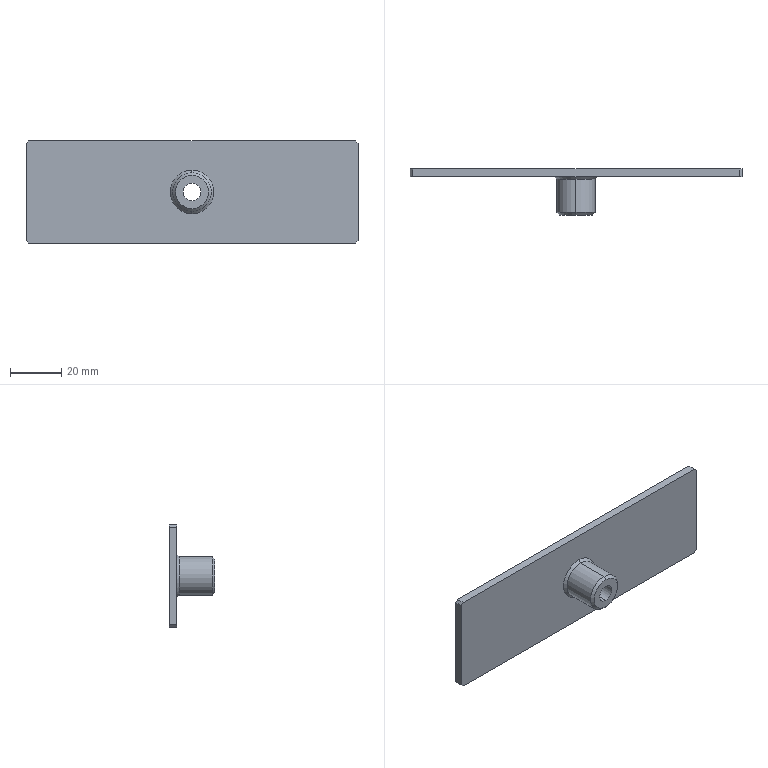Part | SolidWorks | features Chamfer 1, Extrusion 1, HoleWzd 1, ICE 1 | 1 solid | 19 faces | box 130 x 18 x 40 mm | volume 17593 mm3 | plane 11 | cone 4 | cylinder 4 | commonest cylinder face diameters 6.8 x2 15 x2
STEP:
#1=CARTESIAN_POINT('',(0.,0.,-6.5));
#2=VERTEX_POINT('',#1);
#3=CARTESIAN_POINT('',(0.,0.,6.5));
#4=VERTEX_POINT('',#3);
#5=CARTESIAN_POINT('',(0.,0.,0.));
#6=DIRECTION('',(0.,-1.,0.));
#7=DIRECTION('',(0.,0.,1.));
#8=AXIS2_PLACEMENT_3D('',#5,#6,#7);
#9=CIRCLE('',#8,6.5);
#10=EDGE_CURVE('',#2,#4,#9,.T.);
#11=ORIENTED_EDGE('',*,*,#10,.F.);
#12=CARTESIAN_POINT('',(0.,1.,-7.5));
#13=VERTEX_POINT('',#12);
#14=CARTESIAN_POINT('',(0.,1.,-7.5));
#15=DIRECTION('',(0.,0.7071,-0.7071));
#16=VECTOR('',#15,1000.);
#17=LINE('',#14,#16);
#18=EDGE_CURVE('',#2,#13,#17,.T.);
#19=ORIENTED_EDGE('',*,*,#18,.T.);
#20=CARTESIAN_POINT('',(0.,1.,7.5));
#21=VERTEX_POINT('',#20);
#22=CARTESIAN_POINT('',(0.,1.,0.));
#23=DIRECTION('',(0.,1.,0.));
#24=DIRECTION('',(0.,0.,1.));
#25=AXIS2_PLACEMENT_3D('',#22,#23,#24);
#26=CIRCLE('',#25,7.5);
#27=EDGE_CURVE('',#21,#13,#26,.T.);
#28=ORIENTED_EDGE('',*,*,#27,.F.);
#29=CARTESIAN_POINT('',(0.,1.,7.5));
#30=DIRECTION('',(0.,0.7071,0.7071));
#31=VECTOR('',#30,1000.);
#32=LINE('',#29,#31);
#33=EDGE_CURVE('',#4,#21,#32,.T.);
#34=ORIENTED_EDGE('',*,*,#33,.F.);
#35=EDGE_LOOP('',(#11,#19,#28,#34));
#36=FACE_OUTER_BOUND('',#35,.T.);
#37=CARTESIAN_POINT('',(0.,1.,0.));
#38=DIRECTION('',(0.,1.,0.));
#39=DIRECTION('',(0.,0.,1.));
#40=AXIS2_PLACEMENT_3D('',#37,#38,#39);
#41=CONICAL_SURFACE('',#40,7.5,0.7854);
#42=ADVANCED_FACE('',(#36),#41,.T.);
#43=CARTESIAN_POINT('',(0.,14.,-7.5));
#44=VERTEX_POINT('',#43);
#45=CARTESIAN_POINT('',(0.,14.,7.5));
#46=VERTEX_POINT('',#45);
#47=CARTESIAN_POINT('',(0.,14.,0.));
#48=DIRECTION('',(0.,-1.,0.));
#49=DIRECTION('',(0.,0.,1.));
#50=AXIS2_PLACEMENT_3D('',#47,#48,#49);
#51=CIRCLE('',#50,7.5);
#52=EDGE_CURVE('',#44,#46,#51,.T.);
#53=ORIENTED_EDGE('',*,*,#52,.F.);
#54=CARTESIAN_POINT('',(0.,15.,-8.5));
#55=VERTEX_POINT('',#54);
#56=CARTESIAN_POINT('',(0.,15.,-8.5));
#57=DIRECTION('',(0.,0.7071,-0.7071));
#58=VECTOR('',#57,1000.);
#59=LINE('',#56,#58);
#60=EDGE_CURVE('',#44,#55,#59,.T.);
#61=ORIENTED_EDGE('',*,*,#60,.T.);
#62=CARTESIAN_POINT('',(0.,15.,8.5));
#63=VERTEX_POINT('',#62);
#64=CARTESIAN_POINT('',(0.,15.,0.));
#65=DIRECTION('',(0.,1.,0.));
#66=DIRECTION('',(0.,0.,1.));
#67=AXIS2_PLACEMENT_3D('',#64,#65,#66);
#68=CIRCLE('',#67,8.5);
#69=EDGE_CURVE('',#63,#55,#68,.T.);
#70=ORIENTED_EDGE('',*,*,#69,.F.);
#71=CARTESIAN_POINT('',(0.,15.,8.5));
#72=DIRECTION('',(0.,0.7071,0.7071));
#73=VECTOR('',#72,1000.);
#74=LINE('',#71,#73);
#75=EDGE_CURVE('',#46,#63,#74,.T.);
#76=ORIENTED_EDGE('',*,*,#75,.F.);
#77=EDGE_LOOP('',(#53,#61,#70,#76));
#78=FACE_OUTER_BOUND('',#77,.T.);
#79=CARTESIAN_POINT('',(0.,15.,0.));
#80=DIRECTION('',(0.,1.,0.));
#81=DIRECTION('',(0.,0.,1.));
#82=AXIS2_PLACEMENT_3D('',#79,#80,#81);
#83=CONICAL_SURFACE('',#82,8.5,0.7854);
#84=ADVANCED_FACE('',(#78),#83,.T.);
#85=CARTESIAN_POINT('',(0.,18.,-3.4));
#86=VERTEX_POINT('',#85);
#87=CARTESIAN_POINT('',(0.,18.,3.4));
#88=VERTEX_POINT('',#87);
#89=CARTESIAN_POINT('',(0.,18.,0.));
#90=DIRECTION('',(0.,1.,0.));
#91=DIRECTION('',(0.,0.,1.));
#92=AXIS2_PLACEMENT_3D('',#89,#90,#91);
#93=CIRCLE('',#92,3.4);
#94=EDGE_CURVE('',#86,#88,#93,.T.);
#95=ORIENTED_EDGE('',*,*,#94,.T.);
#96=CARTESIAN_POINT('',(0.,0.,3.4));
#97=VERTEX_POINT('',#96);
#98=CARTESIAN_POINT('',(0.,0.,3.4));
#99=DIRECTION('',(0.,-1.,0.));
#100=VECTOR('',#99,1000.);
#101=LINE('',#98,#100);
#102=EDGE_CURVE('',#88,#97,#101,.T.);
#103=ORIENTED_EDGE('',*,*,#102,.T.);
#104=CARTESIAN_POINT('',(0.,0.,-3.4));
#105=VERTEX_POINT('',#104);
#106=CARTESIAN_POINT('',(0.,0.,0.));
#107=DIRECTION('',(0.,-1.,0.));
#108=DIRECTION('',(0.,0.,-1.));
#109=AXIS2_PLACEMENT_3D('',#106,#107,#108);
#110=CIRCLE('',#109,3.4);
#111=EDGE_CURVE('',#97,#105,#110,.T.);
#112=ORIENTED_EDGE('',*,*,#111,.T.);
#113=CARTESIAN_POINT('',(0.,0.,-3.4));
#114=DIRECTION('',(0.,-1.,0.));
#115=VECTOR('',#114,1000.);
#116=LINE('',#113,#115);
#117=EDGE_CURVE('',#86,#105,#116,.T.);
#118=ORIENTED_EDGE('',*,*,#117,.F.);
#119=EDGE_LOOP('',(#95,#103,#112,#118));
#120=FACE_OUTER_BOUND('',#119,.T.);
#121=CARTESIAN_POINT('',(0.,0.,0.));
#122=DIRECTION('',(0.,-1.,0.));
#123=DIRECTION('',(0.,0.,-1.));
#124=AXIS2_PLACEMENT_3D('',#121,#122,#123);
#125=CYLINDRICAL_SURFACE('',#124,3.4);
#126=ADVANCED_FACE('',(#120),#125,.F.);
#127=ORIENTED_EDGE('',*,*,#52,.T.);
#128=CARTESIAN_POINT('',(0.,15.,7.5));
#129=DIRECTION('',(0.,-1.,0.));
#130=VECTOR('',#129,1000.);
#131=LINE('',#128,#130);
#132=EDGE_CURVE('',#46,#21,#131,.T.);
#133=ORIENTED_EDGE('',*,*,#132,.T.);
#134=ORIENTED_EDGE('',*,*,#27,.T.);
#135=CARTESIAN_POINT('',(0.,15.,-7.5));
#136=DIRECTION('',(0.,-1.,0.));
#137=VECTOR('',#136,1000.);
#138=LINE('',#135,#137);
#139=EDGE_CURVE('',#44,#13,#138,.T.);
#140=ORIENTED_EDGE('',*,*,#139,.F.);
#141=EDGE_LOOP('',(#127,#133,#134,#140));
#142=FACE_OUTER_BOUND('',#141,.T.);
#143=CARTESIAN_POINT('',(0.,15.,0.));
#144=DIRECTION('',(0.,-1.,0.));
#145=DIRECTION('',(0.,0.,-1.));
#146=AXIS2_PLACEMENT_3D('',#143,#144,#145);
#147=CYLINDRICAL_SURFACE('',#146,7.5);
#148=ADVANCED_FACE('',(#142),#147,.T.);
#149=ORIENTED_EDGE('',*,*,#132,.F.);
#150=CARTESIAN_POINT('',(0.,14.,0.));
#151=DIRECTION('',(0.,-1.,0.));
#152=DIRECTION('',(0.,0.,1.));
#153=AXIS2_PLACEMENT_3D('',#150,#151,#152);
#154=CIRCLE('',#153,7.5);
#155=EDGE_CURVE('',#46,#44,#154,.T.);
#156=ORIENTED_EDGE('',*,*,#155,.T.);
#157=ORIENTED_EDGE('',*,*,#139,.T.);
#158=CARTESIAN_POINT('',(0.,1.,0.));
#159=DIRECTION('',(0.,1.,0.));
#160=DIRECTION('',(0.,0.,1.));
#161=AXIS2_PLACEMENT_3D('',#158,#159,#160);
#162=CIRCLE('',#161,7.5);
#163=EDGE_CURVE('',#13,#21,#162,.T.);
#164=ORIENTED_EDGE('',*,*,#163,.T.);
#165=EDGE_LOOP('',(#149,#156,#157,#164));
#166=FACE_OUTER_BOUND('',#165,.T.);
#167=CARTESIAN_POINT('',(0.,15.,0.));
#168=DIRECTION('',(0.,-1.,0.));
#169=DIRECTION('',(0.,0.,-1.));
#170=AXIS2_PLACEMENT_3D('',#167,#168,#169);
#171=CYLINDRICAL_SURFACE('',#170,7.5);
#172=ADVANCED_FACE('',(#166),#171,.T.);
#173=CARTESIAN_POINT('',(0.,0.,0.));
#174=DIRECTION('',(0.,-1.,0.));
#175=DIRECTION('',(0.,0.,1.));
#176=AXIS2_PLACEMENT_3D('',#173,#174,#175);
#177=CIRCLE('',#176,6.5);
#178=EDGE_CURVE('',#4,#2,#177,.T.);
#179=ORIENTED_EDGE('',*,*,#178,.T.);
#180=ORIENTED_EDGE('',*,*,#10,.T.);
#181=EDGE_LOOP('',(#179,#180));
#182=FACE_OUTER_BOUND('',#181,.T.);
#183=CARTESIAN_POINT('',(0.,0.,0.));
#184=DIRECTION('',(0.,-1.,0.));
#185=DIRECTION('',(0.,0.,-1.));
#186=AXIS2_PLACEMENT_3D('',#183,#184,#185);
#187=CIRCLE('',#186,3.4);
#188=EDGE_CURVE('',#105,#97,#187,.T.);
#189=ORIENTED_EDGE('',*,*,#188,.F.);
#190=ORIENTED_EDGE('',*,*,#111,.F.);
#191=EDGE_LOOP('',(#189,#190));
#192=FACE_BOUND('',#191,.T.);
#193=CARTESIAN_POINT('',(0.,0.,0.));
#194=DIRECTION('',(0.,1.,0.));
#195=DIRECTION('',(0.,0.,1.));
#196=AXIS2_PLACEMENT_3D('',#193,#194,#195);
#197=PLANE('',#196);
#198=ADVANCED_FACE('',(#182,#192),#197,.F.);
#199=CARTESIAN_POINT('',(65.,15.,19.));
#200=VERTEX_POINT('',#199);
#201=CARTESIAN_POINT('',(65.,15.,-19.));
#202=VERTEX_POINT('',#201);
#203=CARTESIAN_POINT('',(65.,15.,-20.));
#204=DIRECTION('',(0.,0.,-1.));
#205=VECTOR('',#204,1000.);
#206=LINE('',#203,#205);
#207=EDGE_CURVE('',#200,#202,#206,.T.);
#208=ORIENTED_EDGE('',*,*,#207,.T.);
#209=CARTESIAN_POINT('',(65.,18.,-19.));
#210=VERTEX_POINT('',#209);
#211=CARTESIAN_POINT('',(65.,18.,-19.));
#212=DIRECTION('',(0.,1.,0.));
#213=VECTOR('',#212,1000.);
#214=LINE('',#211,#213);
#215=EDGE_CURVE('',#202,#210,#214,.T.);
#216=ORIENTED_EDGE('',*,*,#215,.T.);
#217=CARTESIAN_POINT('',(65.,18.,19.));
#218=VERTEX_POINT('',#217);
#219=CARTESIAN_POINT('',(65.,18.,-20.));
#220=DIRECTION('',(0.,0.,-1.));
#221=VECTOR('',#220,1000.);
#222=LINE('',#219,#221);
#223=EDGE_CURVE('',#218,#210,#222,.T.);
#224=ORIENTED_EDGE('',*,*,#223,.F.);
#225=CARTESIAN_POINT('',(65.,18.,19.));
#226=DIRECTION('',(0.,-1.,0.));
#227=VECTOR('',#226,1000.);
#228=LINE('',#225,#227);
#229=EDGE_CURVE('',#218,#200,#228,.T.);
#230=ORIENTED_EDGE('',*,*,#229,.T.);
#231=EDGE_LOOP('',(#208,#216,#224,#230));
#232=FACE_OUTER_BOUND('',#231,.T.);
#233=CARTESIAN_POINT('',(65.,18.,-20.));
#234=DIRECTION('',(-1.,0.,0.));
#235=DIRECTION('',(0.,0.,1.));
#236=AXIS2_PLACEMENT_3D('',#233,#234,#235);
#237=PLANE('',#236);
#238=ADVANCED_FACE('',(#232),#237,.F.);
#239=CARTESIAN_POINT('',(64.,18.,-20.));
#240=VERTEX_POINT('',#239);
#241=CARTESIAN_POINT('',(-64.,18.,-20.));
#242=VERTEX_POINT('',#241);
#243=CARTESIAN_POINT('',(-65.,18.,-20.));
#244=DIRECTION('',(-1.,0.,0.));
#245=VECTOR('',#244,1000.);
#246=LINE('',#243,#245);
#247=EDGE_CURVE('',#240,#242,#246,.T.);
#248=ORIENTED_EDGE('',*,*,#247,.F.);
#249=CARTESIAN_POINT('',(64.,15.,-20.));
#250=VERTEX_POINT('',#249);
#251=CARTESIAN_POINT('',(64.,18.,-20.));
#252=DIRECTION('',(0.,-1.,0.));
#253=VECTOR('',#252,1000.);
#254=LINE('',#251,#253);
#255=EDGE_CURVE('',#240,#250,#254,.T.);
#256=ORIENTED_EDGE('',*,*,#255,.T.);
#257=CARTESIAN_POINT('',(-64.,15.,-20.));
#258=VERTEX_POINT('',#257);
#259=CARTESIAN_POINT('',(-65.,15.,-20.));
#260=DIRECTION('',(-1.,0.,0.));
#261=VECTOR('',#260,1000.);
#262=LINE('',#259,#261);
#263=EDGE_CURVE('',#250,#258,#262,.T.);
#264=ORIENTED_EDGE('',*,*,#263,.T.);
#265=CARTESIAN_POINT('',(-64.,18.,-20.));
#266=DIRECTION('',(0.,1.,0.));
#267=VECTOR('',#266,1000.);
#268=LINE('',#265,#267);
#269=EDGE_CURVE('',#258,#242,#268,.T.);
#270=ORIENTED_EDGE('',*,*,#269,.T.);
#271=EDGE_LOOP('',(#248,#256,#264,#270));
#272=FACE_OUTER_BOUND('',#271,.T.);
#273=CARTESIAN_POINT('',(-65.,18.,-20.));
#274=DIRECTION('',(0.,0.,1.));
#275=DIRECTION('',(1.,0.,0.));
#276=AXIS2_PLACEMENT_3D('',#273,#274,#275);
#277=PLANE('',#276);
#278=ADVANCED_FACE('',(#272),#277,.F.);
#279=CARTESIAN_POINT('',(-65.,15.,-19.));
#280=VERTEX_POINT('',#279);
#281=CARTESIAN_POINT('',(-65.,15.,19.));
#282=VERTEX_POINT('',#281);
#283=CARTESIAN_POINT('',(-65.,15.,-20.));
#284=DIRECTION('',(0.,0.,1.));
#285=VECTOR('',#284,1000.);
#286=LINE('',#283,#285);
#287=EDGE_CURVE('',#280,#282,#286,.T.);
#288=ORIENTED_EDGE('',*,*,#287,.T.);
#289=CARTESIAN_POINT('',(-65.,18.,19.));
#290=VERTEX_POINT('',#289);
#291=CARTESIAN_POINT('',(-65.,18.,19.));
#292=DIRECTION('',(0.,1.,0.));
#293=VECTOR('',#292,1000.);
#294=LINE('',#291,#293);
#295=EDGE_CURVE('',#282,#290,#294,.T.);
#296=ORIENTED_EDGE('',*,*,#295,.T.);
#297=CARTESIAN_POINT('',(-65.,18.,-19.));
#298=VERTEX_POINT('',#297);
#299=CARTESIAN_POINT('',(-65.,18.,-20.));
#300=DIRECTION('',(0.,0.,1.));
#301=VECTOR('',#300,1000.);
#302=LINE('',#299,#301);
#303=EDGE_CURVE('',#298,#290,#302,.T.);
#304=ORIENTED_EDGE('',*,*,#303,.F.);
#305=CARTESIAN_POINT('',(-65.,18.,-19.));
#306=DIRECTION('',(0.,-1.,0.));
#307=VECTOR('',#306,1000.);
#308=LINE('',#305,#307);
#309=EDGE_CURVE('',#298,#280,#308,.T.);
#310=ORIENTED_EDGE('',*,*,#309,.T.);
#311=EDGE_LOOP('',(#288,#296,#304,#310));
#312=FACE_OUTER_BOUND('',#311,.T.);
#313=CARTESIAN_POINT('',(-65.,18.,-20.));
#314=DIRECTION('',(1.,0.,0.));
#315=DIRECTION('',(0.,0.,-1.));
#316=AXIS2_PLACEMENT_3D('',#313,#314,#315);
#317=PLANE('',#316);
#318=ADVANCED_FACE('',(#312),#317,.F.);
#319=CARTESIAN_POINT('',(-64.,15.,20.));
#320=VERTEX_POINT('',#319);
#321=CARTESIAN_POINT('',(64.,15.,20.));
#322=VERTEX_POINT('',#321);
#323=CARTESIAN_POINT('',(-65.,15.,20.));
#324=DIRECTION('',(1.,0.,0.));
#325=VECTOR('',#324,1000.);
#326=LINE('',#323,#325);
#327=EDGE_CURVE('',#320,#322,#326,.T.);
#328=ORIENTED_EDGE('',*,*,#327,.T.);
#329=CARTESIAN_POINT('',(64.,18.,20.));
#330=VERTEX_POINT('',#329);
#331=CARTESIAN_POINT('',(64.,18.,20.));
#332=DIRECTION('',(0.,1.,0.));
#333=VECTOR('',#332,1000.);
#334=LINE('',#331,#333);
#335=EDGE_CURVE('',#322,#330,#334,.T.);
#336=ORIENTED_EDGE('',*,*,#335,.T.);
#337=CARTESIAN_POINT('',(-64.,18.,20.));
#338=VERTEX_POINT('',#337);
#339=CARTESIAN_POINT('',(-65.,18.,20.));
#340=DIRECTION('',(1.,0.,0.));
#341=VECTOR('',#340,1000.);
#342=LINE('',#339,#341);
#343=EDGE_CURVE('',#338,#330,#342,.T.);
#344=ORIENTED_EDGE('',*,*,#343,.F.);
#345=CARTESIAN_POINT('',(-64.,18.,20.));
#346=DIRECTION('',(0.,-1.,0.));
#347=VECTOR('',#346,1000.);
#348=LINE('',#345,#347);
#349=EDGE_CURVE('',#338,#320,#348,.T.);
#350=ORIENTED_EDGE('',*,*,#349,.T.);
#351=EDGE_LOOP('',(#328,#336,#344,#350));
#352=FACE_OUTER_BOUND('',#351,.T.);
#353=CARTESIAN_POINT('',(-65.,18.,20.));
#354=DIRECTION('',(0.,0.,-1.));
#355=DIRECTION('',(-1.,0.,0.));
#356=AXIS2_PLACEMENT_3D('',#353,#354,#355);
#357=PLANE('',#356);
#358=ADVANCED_FACE('',(#352),#357,.F.);
#359=ORIENTED_EDGE('',*,*,#94,.F.);
#360=CARTESIAN_POINT('',(0.,18.,0.));
#361=DIRECTION('',(0.,1.,0.));
#362=DIRECTION('',(0.,0.,1.));
#363=AXIS2_PLACEMENT_3D('',#360,#361,#362);
#364=CIRCLE('',#363,3.4);
#365=EDGE_CURVE('',#88,#86,#364,.T.);
#366=ORIENTED_EDGE('',*,*,#365,.F.);
#367=EDGE_LOOP('',(#359,#366));
#368=FACE_BOUND('',#367,.T.);
#369=ORIENTED_EDGE('',*,*,#223,.T.);
#370=CARTESIAN_POINT('',(42.,18.,-42.));
#371=DIRECTION('',(-0.7071,0.,-0.7071));
#372=VECTOR('',#371,1000.);
#373=LINE('',#370,#372);
#374=EDGE_CURVE('',#210,#240,#373,.T.);
#375=ORIENTED_EDGE('',*,*,#374,.T.);
#376=ORIENTED_EDGE('',*,*,#247,.T.);
#377=CARTESIAN_POINT('',(-42.,18.,-42.));
#378=DIRECTION('',(-0.7071,0.,0.7071));
#379=VECTOR('',#378,1000.);
#380=LINE('',#377,#379);
#381=EDGE_CURVE('',#242,#298,#380,.T.);
#382=ORIENTED_EDGE('',*,*,#381,.T.);
#383=ORIENTED_EDGE('',*,*,#303,.T.);
#384=CARTESIAN_POINT('',(-42.,18.,42.));
#385=DIRECTION('',(0.7071,0.,0.7071));
#386=VECTOR('',#385,1000.);
#387=LINE('',#384,#386);
#388=EDGE_CURVE('',#290,#338,#387,.T.);
#389=ORIENTED_EDGE('',*,*,#388,.T.);
#390=ORIENTED_EDGE('',*,*,#343,.T.);
#391=CARTESIAN_POINT('',(42.,18.,42.));
#392=DIRECTION('',(0.7071,0.,-0.7071));
#393=VECTOR('',#392,1000.);
#394=LINE('',#391,#393);
#395=EDGE_CURVE('',#330,#218,#394,.T.);
#396=ORIENTED_EDGE('',*,*,#395,.T.);
#397=EDGE_LOOP('',(#369,#375,#376,#382,#383,#389,#390,#396));
#398=FACE_OUTER_BOUND('',#397,.T.);
#399=CARTESIAN_POINT('',(0.,18.,0.));
#400=DIRECTION('',(0.,1.,0.));
#401=DIRECTION('',(0.,0.,1.));
#402=AXIS2_PLACEMENT_3D('',#399,#400,#401);
#403=PLANE('',#402);
#404=ADVANCED_FACE('',(#368,#398),#403,.T.);
#405=ORIENTED_EDGE('',*,*,#69,.T.);
#406=CARTESIAN_POINT('',(0.,15.,0.));
#407=DIRECTION('',(0.,1.,0.));
#408=DIRECTION('',(0.,0.,1.));
#409=AXIS2_PLACEMENT_3D('',#406,#407,#408);
#410=CIRCLE('',#409,8.5);
#411=EDGE_CURVE('',#55,#63,#410,.T.);
#412=ORIENTED_EDGE('',*,*,#411,.T.);
#413=EDGE_LOOP('',(#405,#412));
#414=FACE_BOUND('',#413,.T.);
#415=ORIENTED_EDGE('',*,*,#263,.F.);
#416=CARTESIAN_POINT('',(64.,15.,-20.));
#417=DIRECTION('',(0.7071,0.,0.7071));
#418=VECTOR('',#417,1000.);
#419=LINE('',#416,#418);
#420=EDGE_CURVE('',#250,#202,#419,.T.);
#421=ORIENTED_EDGE('',*,*,#420,.T.);
#422=ORIENTED_EDGE('',*,*,#207,.F.);
#423=CARTESIAN_POINT('',(65.,15.,19.));
#424=DIRECTION('',(-0.7071,0.,0.7071));
#425=VECTOR('',#424,1000.);
#426=LINE('',#423,#425);
#427=EDGE_CURVE('',#200,#322,#426,.T.);
#428=ORIENTED_EDGE('',*,*,#427,.T.);
#429=ORIENTED_EDGE('',*,*,#327,.F.);
#430=CARTESIAN_POINT('',(-64.,15.,20.));
#431=DIRECTION('',(-0.7071,0.,-0.7071));
#432=VECTOR('',#431,1000.);
#433=LINE('',#430,#432);
#434=EDGE_CURVE('',#320,#282,#433,.T.);
#435=ORIENTED_EDGE('',*,*,#434,.T.);
#436=ORIENTED_EDGE('',*,*,#287,.F.);
#437=CARTESIAN_POINT('',(-65.,15.,-19.));
#438=DIRECTION('',(0.7071,0.,-0.7071));
#439=VECTOR('',#438,1000.);
#440=LINE('',#437,#439);
#441=EDGE_CURVE('',#280,#258,#440,.T.);
#442=ORIENTED_EDGE('',*,*,#441,.T.);
#443=EDGE_LOOP('',(#415,#421,#422,#428,#429,#435,#436,#442));
#444=FACE_OUTER_BOUND('',#443,.T.);
#445=CARTESIAN_POINT('',(0.,15.,0.));
#446=DIRECTION('',(0.,1.,0.));
#447=DIRECTION('',(0.,0.,1.));
#448=AXIS2_PLACEMENT_3D('',#445,#446,#447);
#449=PLANE('',#448);
#450=ADVANCED_FACE('',(#414,#444),#449,.F.);
#451=ORIENTED_EDGE('',*,*,#102,.F.);
#452=ORIENTED_EDGE('',*,*,#365,.T.);
#453=ORIENTED_EDGE('',*,*,#117,.T.);
#454=ORIENTED_EDGE('',*,*,#188,.T.);
#455=EDGE_LOOP('',(#451,#452,#453,#454));
#456=FACE_OUTER_BOUND('',#455,.T.);
#457=CARTESIAN_POINT('',(0.,0.,0.));
#458=DIRECTION('',(0.,-1.,0.));
#459=DIRECTION('',(0.,0.,-1.));
#460=AXIS2_PLACEMENT_3D('',#457,#458,#459);
#461=CYLINDRICAL_SURFACE('',#460,3.4);
#462=ADVANCED_FACE('',(#456),#461,.F.);
#463=ORIENTED_EDGE('',*,*,#60,.F.);
#464=ORIENTED_EDGE('',*,*,#155,.F.);
#465=ORIENTED_EDGE('',*,*,#75,.T.);
#466=ORIENTED_EDGE('',*,*,#411,.F.);
#467=EDGE_LOOP('',(#463,#464,#465,#466));
#468=FACE_OUTER_BOUND('',#467,.T.);
#469=CARTESIAN_POINT('',(0.,15.,0.));
#470=DIRECTION('',(0.,1.,0.));
#471=DIRECTION('',(0.,0.,1.));
#472=AXIS2_PLACEMENT_3D('',#469,#470,#471);
#473=CONICAL_SURFACE('',#472,8.5,0.7854);
#474=ADVANCED_FACE('',(#468),#473,.T.);
#475=ORIENTED_EDGE('',*,*,#18,.F.);
#476=ORIENTED_EDGE('',*,*,#178,.F.);
#477=ORIENTED_EDGE('',*,*,#33,.T.);
#478=ORIENTED_EDGE('',*,*,#163,.F.);
#479=EDGE_LOOP('',(#475,#476,#477,#478));
#480=FACE_OUTER_BOUND('',#479,.T.);
#481=CARTESIAN_POINT('',(0.,1.,0.));
#482=DIRECTION('',(0.,1.,0.));
#483=DIRECTION('',(0.,0.,1.));
#484=AXIS2_PLACEMENT_3D('',#481,#482,#483);
#485=CONICAL_SURFACE('',#484,7.5,0.7854);
#486=ADVANCED_FACE('',(#480),#485,.T.);
#487=ORIENTED_EDGE('',*,*,#374,.F.);
#488=ORIENTED_EDGE('',*,*,#215,.F.);
#489=ORIENTED_EDGE('',*,*,#420,.F.);
#490=ORIENTED_EDGE('',*,*,#255,.F.);
#491=EDGE_LOOP('',(#487,#488,#489,#490));
#492=FACE_OUTER_BOUND('',#491,.T.);
#493=CARTESIAN_POINT('',(64.,18.,-20.));
#494=DIRECTION('',(-0.7071,0.,0.7071));
#495=DIRECTION('',(0.,-1.,0.));
#496=AXIS2_PLACEMENT_3D('',#493,#494,#495);
#497=PLANE('',#496);
#498=ADVANCED_FACE('',(#492),#497,.F.);
#499=ORIENTED_EDGE('',*,*,#395,.F.);
#500=ORIENTED_EDGE('',*,*,#335,.F.);
#501=ORIENTED_EDGE('',*,*,#427,.F.);
#502=ORIENTED_EDGE('',*,*,#229,.F.);
#503=EDGE_LOOP('',(#499,#500,#501,#502));
#504=FACE_OUTER_BOUND('',#503,.T.);
#505=CARTESIAN_POINT('',(65.,18.,19.));
#506=DIRECTION('',(-0.7071,0.,-0.7071));
#507=DIRECTION('',(0.,-1.,0.));
#508=AXIS2_PLACEMENT_3D('',#505,#506,#507);
#509=PLANE('',#508);
#510=ADVANCED_FACE('',(#504),#509,.F.);
#511=ORIENTED_EDGE('',*,*,#388,.F.);
#512=ORIENTED_EDGE('',*,*,#295,.F.);
#513=ORIENTED_EDGE('',*,*,#434,.F.);
#514=ORIENTED_EDGE('',*,*,#349,.F.);
#515=EDGE_LOOP('',(#511,#512,#513,#514));
#516=FACE_OUTER_BOUND('',#515,.T.);
#517=CARTESIAN_POINT('',(-64.,18.,20.));
#518=DIRECTION('',(0.7071,0.,-0.7071));
#519=DIRECTION('',(0.,-1.,0.));
#520=AXIS2_PLACEMENT_3D('',#517,#518,#519);
#521=PLANE('',#520);
#522=ADVANCED_FACE('',(#516),#521,.F.);
#523=ORIENTED_EDGE('',*,*,#381,.F.);
#524=ORIENTED_EDGE('',*,*,#269,.F.);
#525=ORIENTED_EDGE('',*,*,#441,.F.);
#526=ORIENTED_EDGE('',*,*,#309,.F.);
#527=EDGE_LOOP('',(#523,#524,#525,#526));
#528=FACE_OUTER_BOUND('',#527,.T.);
#529=CARTESIAN_POINT('',(-65.,18.,-19.));
#530=DIRECTION('',(0.7071,0.,0.7071));
#531=DIRECTION('',(0.,-1.,0.));
#532=AXIS2_PLACEMENT_3D('',#529,#530,#531);
#533=PLANE('',#532);
#534=ADVANCED_FACE('',(#528),#533,.F.);
#535=CLOSED_SHELL('',(#42,#84,#126,#148,#172,#198,#238,#278,#318,#358,#404,#450,#462,#474,#486,#498,#510,#522,#534));
#536=MANIFOLD_SOLID_BREP('',#535);
#537=CARTESIAN_POINT('',(0.,0.,0.));
#538=DIRECTION('',(0.,0.,1.));
#539=DIRECTION('',(1.,0.,0.));
#540=AXIS2_PLACEMENT_3D('',#537,#538,#539);
#541=(LENGTH_UNIT()NAMED_UNIT(*)SI_UNIT(.MILLI.,.METRE.));
#542=UNCERTAINTY_MEASURE_WITH_UNIT(LENGTH_MEASURE(0.00001),#541,'','');
#543=(NAMED_UNIT(*)PLANE_ANGLE_UNIT()SI_UNIT($,.RADIAN.));
#544=(NAMED_UNIT(*)SI_UNIT($,.STERADIAN.)SOLID_ANGLE_UNIT());
#545=(GEOMETRIC_REPRESENTATION_CONTEXT(3)GLOBAL_UNCERTAINTY_ASSIGNED_CONTEXT((#542))GLOBAL_UNIT_ASSIGNED_CONTEXT((#541,#543,#544))REPRESENTATION_CONTEXT('',''));
#546=ADVANCED_BREP_SHAPE_REPRESENTATION('',(#536,#540),#545);